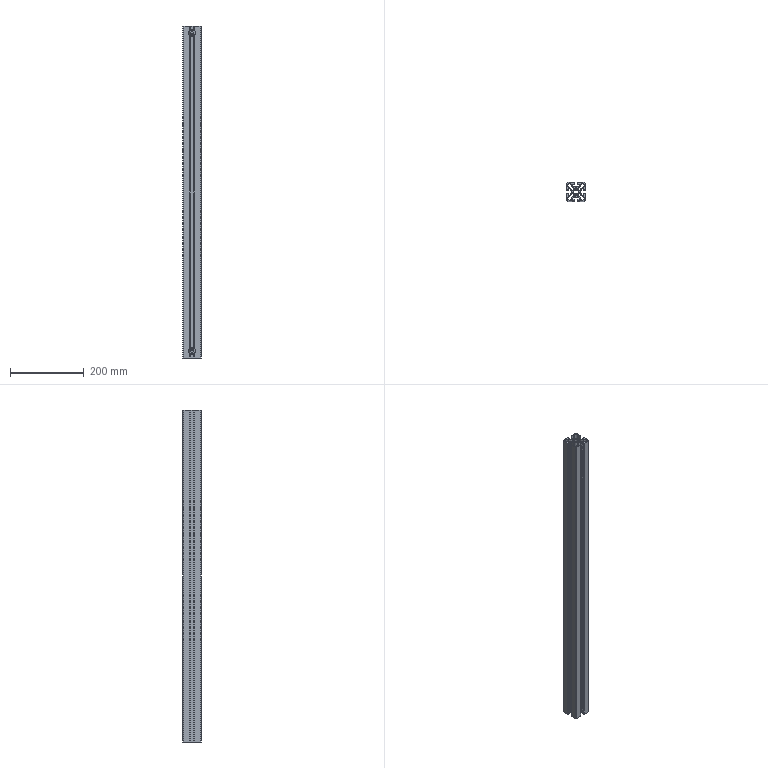Part | NX | features BREP 1 | 1 solid | 252 faces | box 50 x 50 x 900 mm | volume 883893 mm3 | plane 169 | cylinder 83 | commonest cylinder face diameters 2 x39 19 x20 10 x12 6 x4 12 x4 17 x4